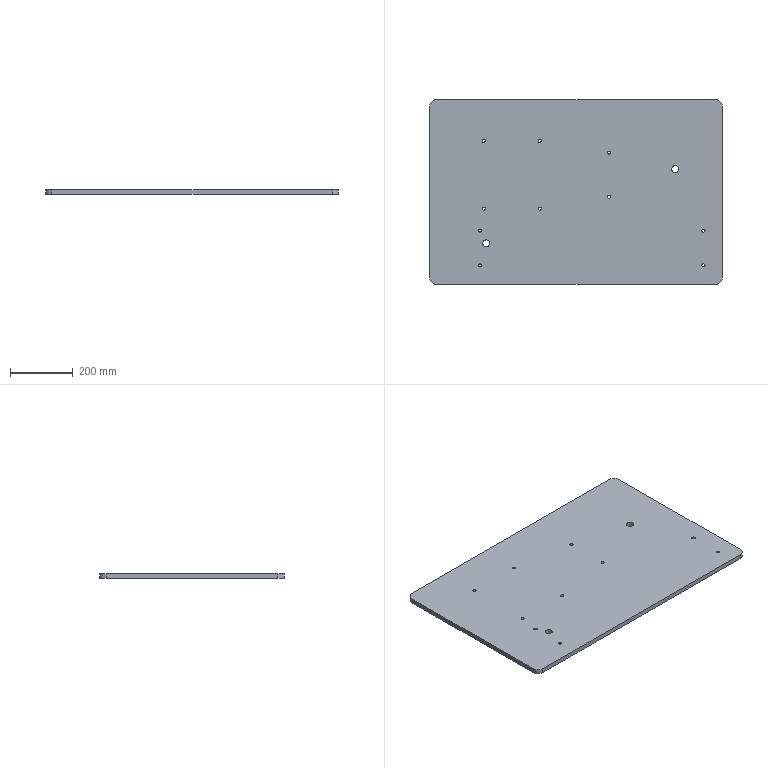Part | SolidWorks | features Extrusion 1 | 1 solid | 34 faces | box 930 x 586 x 15 mm | volume 8146365 mm3 | cylinder 28 | plane 6 | commonest cylinder face diameters 10 x20 22 x4 40 x4
STEP:
#1=CARTESIAN_POINT('',(-296.,-163.,15.));
#2=VERTEX_POINT('',#1);
#3=CARTESIAN_POINT('',(-274.,-163.,15.));
#4=VERTEX_POINT('',#3);
#5=CARTESIAN_POINT('',(-285.,-163.,15.));
#6=DIRECTION('',(0.,0.,1.));
#7=DIRECTION('',(1.,0.,0.));
#8=AXIS2_PLACEMENT_3D('',#5,#6,#7);
#9=CIRCLE('',#8,11.);
#10=EDGE_CURVE('',#2,#4,#9,.T.);
#11=ORIENTED_EDGE('',*,*,#10,.T.);
#12=CARTESIAN_POINT('',(-274.,-163.,0.));
#13=VERTEX_POINT('',#12);
#14=CARTESIAN_POINT('',(-274.,-163.,15.));
#15=DIRECTION('',(0.,0.,-1.));
#16=VECTOR('',#15,1000.);
#17=LINE('',#14,#16);
#18=EDGE_CURVE('',#4,#13,#17,.T.);
#19=ORIENTED_EDGE('',*,*,#18,.T.);
#20=CARTESIAN_POINT('',(-296.,-163.,0.));
#21=VERTEX_POINT('',#20);
#22=CARTESIAN_POINT('',(-285.,-163.,0.));
#23=DIRECTION('',(0.,0.,1.));
#24=DIRECTION('',(1.,0.,0.));
#25=AXIS2_PLACEMENT_3D('',#22,#23,#24);
#26=CIRCLE('',#25,11.);
#27=EDGE_CURVE('',#21,#13,#26,.T.);
#28=ORIENTED_EDGE('',*,*,#27,.F.);
#29=CARTESIAN_POINT('',(-296.,-163.,15.));
#30=DIRECTION('',(0.,0.,-1.));
#31=VECTOR('',#30,1000.);
#32=LINE('',#29,#31);
#33=EDGE_CURVE('',#2,#21,#32,.T.);
#34=ORIENTED_EDGE('',*,*,#33,.F.);
#35=EDGE_LOOP('',(#11,#19,#28,#34));
#36=FACE_OUTER_BOUND('',#35,.T.);
#37=CARTESIAN_POINT('',(-285.,-163.,15.));
#38=DIRECTION('',(0.,0.,-1.));
#39=DIRECTION('',(-1.,0.,0.));
#40=AXIS2_PLACEMENT_3D('',#37,#38,#39);
#41=CYLINDRICAL_SURFACE('',#40,11.);
#42=ADVANCED_FACE('',(#36),#41,.F.);
#43=CARTESIAN_POINT('',(304.,72.5,15.));
#44=VERTEX_POINT('',#43);
#45=CARTESIAN_POINT('',(326.,72.5,15.));
#46=VERTEX_POINT('',#45);
#47=CARTESIAN_POINT('',(315.,72.5,15.));
#48=DIRECTION('',(0.,0.,1.));
#49=DIRECTION('',(1.,0.,0.));
#50=AXIS2_PLACEMENT_3D('',#47,#48,#49);
#51=CIRCLE('',#50,11.);
#52=EDGE_CURVE('',#44,#46,#51,.T.);
#53=ORIENTED_EDGE('',*,*,#52,.T.);
#54=CARTESIAN_POINT('',(326.,72.5,0.));
#55=VERTEX_POINT('',#54);
#56=CARTESIAN_POINT('',(326.,72.5,15.));
#57=DIRECTION('',(0.,0.,-1.));
#58=VECTOR('',#57,1000.);
#59=LINE('',#56,#58);
#60=EDGE_CURVE('',#46,#55,#59,.T.);
#61=ORIENTED_EDGE('',*,*,#60,.T.);
#62=CARTESIAN_POINT('',(304.,72.5,0.));
#63=VERTEX_POINT('',#62);
#64=CARTESIAN_POINT('',(315.,72.5,0.));
#65=DIRECTION('',(0.,0.,1.));
#66=DIRECTION('',(1.,0.,0.));
#67=AXIS2_PLACEMENT_3D('',#64,#65,#66);
#68=CIRCLE('',#67,11.);
#69=EDGE_CURVE('',#63,#55,#68,.T.);
#70=ORIENTED_EDGE('',*,*,#69,.F.);
#71=CARTESIAN_POINT('',(304.,72.5,15.));
#72=DIRECTION('',(0.,0.,-1.));
#73=VECTOR('',#72,1000.);
#74=LINE('',#71,#73);
#75=EDGE_CURVE('',#44,#63,#74,.T.);
#76=ORIENTED_EDGE('',*,*,#75,.F.);
#77=EDGE_LOOP('',(#53,#61,#70,#76));
#78=FACE_OUTER_BOUND('',#77,.T.);
#79=CARTESIAN_POINT('',(315.,72.5,15.));
#80=DIRECTION('',(0.,0.,-1.));
#81=DIRECTION('',(-1.,0.,0.));
#82=AXIS2_PLACEMENT_3D('',#79,#80,#81);
#83=CYLINDRICAL_SURFACE('',#82,11.);
#84=ADVANCED_FACE('',(#78),#83,.F.);
#85=CARTESIAN_POINT('',(400.,-123.,15.));
#86=VERTEX_POINT('',#85);
#87=CARTESIAN_POINT('',(410.,-123.,15.));
#88=VERTEX_POINT('',#87);
#89=CARTESIAN_POINT('',(405.,-123.,15.));
#90=DIRECTION('',(0.,0.,1.));
#91=DIRECTION('',(-1.,0.,0.));
#92=AXIS2_PLACEMENT_3D('',#89,#90,#91);
#93=CIRCLE('',#92,5.);
#94=EDGE_CURVE('',#86,#88,#93,.T.);
#95=ORIENTED_EDGE('',*,*,#94,.T.);
#96=CARTESIAN_POINT('',(410.,-123.,0.));
#97=VERTEX_POINT('',#96);
#98=CARTESIAN_POINT('',(410.,-123.,15.));
#99=DIRECTION('',(0.,0.,-1.));
#100=VECTOR('',#99,1000.);
#101=LINE('',#98,#100);
#102=EDGE_CURVE('',#88,#97,#101,.T.);
#103=ORIENTED_EDGE('',*,*,#102,.T.);
#104=CARTESIAN_POINT('',(400.,-123.,0.));
#105=VERTEX_POINT('',#104);
#106=CARTESIAN_POINT('',(405.,-123.,0.));
#107=DIRECTION('',(0.,0.,1.));
#108=DIRECTION('',(-1.,0.,0.));
#109=AXIS2_PLACEMENT_3D('',#106,#107,#108);
#110=CIRCLE('',#109,5.);
#111=EDGE_CURVE('',#105,#97,#110,.T.);
#112=ORIENTED_EDGE('',*,*,#111,.F.);
#113=CARTESIAN_POINT('',(400.,-123.,15.));
#114=DIRECTION('',(0.,0.,-1.));
#115=VECTOR('',#114,1000.);
#116=LINE('',#113,#115);
#117=EDGE_CURVE('',#86,#105,#116,.T.);
#118=ORIENTED_EDGE('',*,*,#117,.F.);
#119=EDGE_LOOP('',(#95,#103,#112,#118));
#120=FACE_OUTER_BOUND('',#119,.T.);
#121=CARTESIAN_POINT('',(405.,-123.,15.));
#122=DIRECTION('',(0.,0.,-1.));
#123=DIRECTION('',(-1.,0.,0.));
#124=AXIS2_PLACEMENT_3D('',#121,#122,#123);
#125=CYLINDRICAL_SURFACE('',#124,5.);
#126=ADVANCED_FACE('',(#120),#125,.F.);
#127=CARTESIAN_POINT('',(400.,-233.,15.));
#128=VERTEX_POINT('',#127);
#129=CARTESIAN_POINT('',(410.,-233.,15.));
#130=VERTEX_POINT('',#129);
#131=CARTESIAN_POINT('',(405.,-233.,15.));
#132=DIRECTION('',(0.,0.,1.));
#133=DIRECTION('',(1.,0.,0.));
#134=AXIS2_PLACEMENT_3D('',#131,#132,#133);
#135=CIRCLE('',#134,5.);
#136=EDGE_CURVE('',#128,#130,#135,.T.);
#137=ORIENTED_EDGE('',*,*,#136,.T.);
#138=CARTESIAN_POINT('',(410.,-233.,0.));
#139=VERTEX_POINT('',#138);
#140=CARTESIAN_POINT('',(410.,-233.,15.));
#141=DIRECTION('',(0.,0.,-1.));
#142=VECTOR('',#141,1000.);
#143=LINE('',#140,#142);
#144=EDGE_CURVE('',#130,#139,#143,.T.);
#145=ORIENTED_EDGE('',*,*,#144,.T.);
#146=CARTESIAN_POINT('',(400.,-233.,0.));
#147=VERTEX_POINT('',#146);
#148=CARTESIAN_POINT('',(405.,-233.,0.));
#149=DIRECTION('',(0.,0.,1.));
#150=DIRECTION('',(1.,0.,0.));
#151=AXIS2_PLACEMENT_3D('',#148,#149,#150);
#152=CIRCLE('',#151,5.);
#153=EDGE_CURVE('',#147,#139,#152,.T.);
#154=ORIENTED_EDGE('',*,*,#153,.F.);
#155=CARTESIAN_POINT('',(400.,-233.,15.));
#156=DIRECTION('',(0.,0.,-1.));
#157=VECTOR('',#156,1000.);
#158=LINE('',#155,#157);
#159=EDGE_CURVE('',#128,#147,#158,.T.);
#160=ORIENTED_EDGE('',*,*,#159,.F.);
#161=EDGE_LOOP('',(#137,#145,#154,#160));
#162=FACE_OUTER_BOUND('',#161,.T.);
#163=CARTESIAN_POINT('',(405.,-233.,15.));
#164=DIRECTION('',(0.,0.,-1.));
#165=DIRECTION('',(-1.,0.,0.));
#166=AXIS2_PLACEMENT_3D('',#163,#164,#165);
#167=CYLINDRICAL_SURFACE('',#166,5.);
#168=ADVANCED_FACE('',(#162),#167,.F.);
#169=CARTESIAN_POINT('',(-310.,-233.,15.));
#170=VERTEX_POINT('',#169);
#171=CARTESIAN_POINT('',(-300.,-233.,15.));
#172=VERTEX_POINT('',#171);
#173=CARTESIAN_POINT('',(-305.,-233.,15.));
#174=DIRECTION('',(0.,0.,1.));
#175=DIRECTION('',(-1.,0.,0.));
#176=AXIS2_PLACEMENT_3D('',#173,#174,#175);
#177=CIRCLE('',#176,5.);
#178=EDGE_CURVE('',#170,#172,#177,.T.);
#179=ORIENTED_EDGE('',*,*,#178,.T.);
#180=CARTESIAN_POINT('',(-300.,-233.,0.));
#181=VERTEX_POINT('',#180);
#182=CARTESIAN_POINT('',(-300.,-233.,15.));
#183=DIRECTION('',(0.,0.,-1.));
#184=VECTOR('',#183,1000.);
#185=LINE('',#182,#184);
#186=EDGE_CURVE('',#172,#181,#185,.T.);
#187=ORIENTED_EDGE('',*,*,#186,.T.);
#188=CARTESIAN_POINT('',(-310.,-233.,0.));
#189=VERTEX_POINT('',#188);
#190=CARTESIAN_POINT('',(-305.,-233.,0.));
#191=DIRECTION('',(0.,0.,1.));
#192=DIRECTION('',(-1.,0.,0.));
#193=AXIS2_PLACEMENT_3D('',#190,#191,#192);
#194=CIRCLE('',#193,5.);
#195=EDGE_CURVE('',#189,#181,#194,.T.);
#196=ORIENTED_EDGE('',*,*,#195,.F.);
#197=CARTESIAN_POINT('',(-310.,-233.,15.));
#198=DIRECTION('',(0.,0.,-1.));
#199=VECTOR('',#198,1000.);
#200=LINE('',#197,#199);
#201=EDGE_CURVE('',#170,#189,#200,.T.);
#202=ORIENTED_EDGE('',*,*,#201,.F.);
#203=EDGE_LOOP('',(#179,#187,#196,#202));
#204=FACE_OUTER_BOUND('',#203,.T.);
#205=CARTESIAN_POINT('',(-305.,-233.,15.));
#206=DIRECTION('',(0.,0.,-1.));
#207=DIRECTION('',(-1.,0.,0.));
#208=AXIS2_PLACEMENT_3D('',#205,#206,#207);
#209=CYLINDRICAL_SURFACE('',#208,5.);
#210=ADVANCED_FACE('',(#204),#209,.F.);
#211=CARTESIAN_POINT('',(-310.,-123.,15.));
#212=VERTEX_POINT('',#211);
#213=CARTESIAN_POINT('',(-300.,-123.,15.));
#214=VERTEX_POINT('',#213);
#215=CARTESIAN_POINT('',(-305.,-123.,15.));
#216=DIRECTION('',(0.,0.,1.));
#217=DIRECTION('',(1.,0.,0.));
#218=AXIS2_PLACEMENT_3D('',#215,#216,#217);
#219=CIRCLE('',#218,5.);
#220=EDGE_CURVE('',#212,#214,#219,.T.);
#221=ORIENTED_EDGE('',*,*,#220,.T.);
#222=CARTESIAN_POINT('',(-300.,-123.,0.));
#223=VERTEX_POINT('',#222);
#224=CARTESIAN_POINT('',(-300.,-123.,15.));
#225=DIRECTION('',(0.,0.,-1.));
#226=VECTOR('',#225,1000.);
#227=LINE('',#224,#226);
#228=EDGE_CURVE('',#214,#223,#227,.T.);
#229=ORIENTED_EDGE('',*,*,#228,.T.);
#230=CARTESIAN_POINT('',(-310.,-123.,0.));
#231=VERTEX_POINT('',#230);
#232=CARTESIAN_POINT('',(-305.,-123.,0.));
#233=DIRECTION('',(0.,0.,1.));
#234=DIRECTION('',(1.,0.,0.));
#235=AXIS2_PLACEMENT_3D('',#232,#233,#234);
#236=CIRCLE('',#235,5.);
#237=EDGE_CURVE('',#231,#223,#236,.T.);
#238=ORIENTED_EDGE('',*,*,#237,.F.);
#239=CARTESIAN_POINT('',(-310.,-123.,15.));
#240=DIRECTION('',(0.,0.,-1.));
#241=VECTOR('',#240,1000.);
#242=LINE('',#239,#241);
#243=EDGE_CURVE('',#212,#231,#242,.T.);
#244=ORIENTED_EDGE('',*,*,#243,.F.);
#245=EDGE_LOOP('',(#221,#229,#238,#244));
#246=FACE_OUTER_BOUND('',#245,.T.);
#247=CARTESIAN_POINT('',(-305.,-123.,15.));
#248=DIRECTION('',(0.,0.,-1.));
#249=DIRECTION('',(-1.,0.,0.));
#250=AXIS2_PLACEMENT_3D('',#247,#248,#249);
#251=CYLINDRICAL_SURFACE('',#250,5.);
#252=ADVANCED_FACE('',(#246),#251,.F.);
#253=CARTESIAN_POINT('',(100.,-15.,15.));
#254=VERTEX_POINT('',#253);
#255=CARTESIAN_POINT('',(110.,-15.,15.));
#256=VERTEX_POINT('',#255);
#257=CARTESIAN_POINT('',(105.,-15.,15.));
#258=DIRECTION('',(0.,0.,1.));
#259=DIRECTION('',(1.,0.,0.));
#260=AXIS2_PLACEMENT_3D('',#257,#258,#259);
#261=CIRCLE('',#260,5.);
#262=EDGE_CURVE('',#254,#256,#261,.T.);
#263=ORIENTED_EDGE('',*,*,#262,.T.);
#264=CARTESIAN_POINT('',(110.,-15.,0.));
#265=VERTEX_POINT('',#264);
#266=CARTESIAN_POINT('',(110.,-15.,15.));
#267=DIRECTION('',(0.,0.,-1.));
#268=VECTOR('',#267,1000.);
#269=LINE('',#266,#268);
#270=EDGE_CURVE('',#256,#265,#269,.T.);
#271=ORIENTED_EDGE('',*,*,#270,.T.);
#272=CARTESIAN_POINT('',(100.,-15.,0.));
#273=VERTEX_POINT('',#272);
#274=CARTESIAN_POINT('',(105.,-15.,0.));
#275=DIRECTION('',(0.,0.,1.));
#276=DIRECTION('',(1.,0.,0.));
#277=AXIS2_PLACEMENT_3D('',#274,#275,#276);
#278=CIRCLE('',#277,5.);
#279=EDGE_CURVE('',#273,#265,#278,.T.);
#280=ORIENTED_EDGE('',*,*,#279,.F.);
#281=CARTESIAN_POINT('',(100.,-15.,15.));
#282=DIRECTION('',(0.,0.,-1.));
#283=VECTOR('',#282,1000.);
#284=LINE('',#281,#283);
#285=EDGE_CURVE('',#254,#273,#284,.T.);
#286=ORIENTED_EDGE('',*,*,#285,.F.);
#287=EDGE_LOOP('',(#263,#271,#280,#286));
#288=FACE_OUTER_BOUND('',#287,.T.);
#289=CARTESIAN_POINT('',(105.,-15.,15.));
#290=DIRECTION('',(0.,0.,-1.));
#291=DIRECTION('',(-1.,0.,0.));
#292=AXIS2_PLACEMENT_3D('',#289,#290,#291);
#293=CYLINDRICAL_SURFACE('',#292,5.);
#294=ADVANCED_FACE('',(#288),#293,.F.);
#295=CARTESIAN_POINT('',(100.,125.,15.));
#296=VERTEX_POINT('',#295);
#297=CARTESIAN_POINT('',(110.,125.,15.));
#298=VERTEX_POINT('',#297);
#299=CARTESIAN_POINT('',(105.,125.,15.));
#300=DIRECTION('',(0.,0.,1.));
#301=DIRECTION('',(-1.,0.,0.));
#302=AXIS2_PLACEMENT_3D('',#299,#300,#301);
#303=CIRCLE('',#302,5.);
#304=EDGE_CURVE('',#296,#298,#303,.T.);
#305=ORIENTED_EDGE('',*,*,#304,.T.);
#306=CARTESIAN_POINT('',(110.,125.,0.));
#307=VERTEX_POINT('',#306);
#308=CARTESIAN_POINT('',(110.,125.,15.));
#309=DIRECTION('',(0.,0.,-1.));
#310=VECTOR('',#309,1000.);
#311=LINE('',#308,#310);
#312=EDGE_CURVE('',#298,#307,#311,.T.);
#313=ORIENTED_EDGE('',*,*,#312,.T.);
#314=CARTESIAN_POINT('',(100.,125.,0.));
#315=VERTEX_POINT('',#314);
#316=CARTESIAN_POINT('',(105.,125.,0.));
#317=DIRECTION('',(0.,0.,1.));
#318=DIRECTION('',(-1.,0.,0.));
#319=AXIS2_PLACEMENT_3D('',#316,#317,#318);
#320=CIRCLE('',#319,5.);
#321=EDGE_CURVE('',#315,#307,#320,.T.);
#322=ORIENTED_EDGE('',*,*,#321,.F.);
#323=CARTESIAN_POINT('',(100.,125.,15.));
#324=DIRECTION('',(0.,0.,-1.));
#325=VECTOR('',#324,1000.);
#326=LINE('',#323,#325);
#327=EDGE_CURVE('',#296,#315,#326,.T.);
#328=ORIENTED_EDGE('',*,*,#327,.F.);
#329=EDGE_LOOP('',(#305,#313,#322,#328));
#330=FACE_OUTER_BOUND('',#329,.T.);
#331=CARTESIAN_POINT('',(105.,125.,15.));
#332=DIRECTION('',(0.,0.,-1.));
#333=DIRECTION('',(-1.,0.,0.));
#334=AXIS2_PLACEMENT_3D('',#331,#332,#333);
#335=CYLINDRICAL_SURFACE('',#334,5.);
#336=ADVANCED_FACE('',(#330),#335,.F.);
#337=CARTESIAN_POINT('',(-298.,-53.,15.));
#338=VERTEX_POINT('',#337);
#339=CARTESIAN_POINT('',(-288.,-53.,15.));
#340=VERTEX_POINT('',#339);
#341=CARTESIAN_POINT('',(-293.,-53.,15.));
#342=DIRECTION('',(0.,0.,1.));
#343=DIRECTION('',(-1.,0.,0.));
#344=AXIS2_PLACEMENT_3D('',#341,#342,#343);
#345=CIRCLE('',#344,5.);
#346=EDGE_CURVE('',#338,#340,#345,.T.);
#347=ORIENTED_EDGE('',*,*,#346,.T.);
#348=CARTESIAN_POINT('',(-288.,-53.,0.));
#349=VERTEX_POINT('',#348);
#350=CARTESIAN_POINT('',(-288.,-53.,15.));
#351=DIRECTION('',(0.,0.,-1.));
#352=VECTOR('',#351,1000.);
#353=LINE('',#350,#352);
#354=EDGE_CURVE('',#340,#349,#353,.T.);
#355=ORIENTED_EDGE('',*,*,#354,.T.);
#356=CARTESIAN_POINT('',(-298.,-53.,0.));
#357=VERTEX_POINT('',#356);
#358=CARTESIAN_POINT('',(-293.,-53.,0.));
#359=DIRECTION('',(0.,0.,1.));
#360=DIRECTION('',(-1.,0.,0.));
#361=AXIS2_PLACEMENT_3D('',#358,#359,#360);
#362=CIRCLE('',#361,5.);
#363=EDGE_CURVE('',#357,#349,#362,.T.);
#364=ORIENTED_EDGE('',*,*,#363,.F.);
#365=CARTESIAN_POINT('',(-298.,-53.,15.));
#366=DIRECTION('',(0.,0.,-1.));
#367=VECTOR('',#366,1000.);
#368=LINE('',#365,#367);
#369=EDGE_CURVE('',#338,#357,#368,.T.);
#370=ORIENTED_EDGE('',*,*,#369,.F.);
#371=EDGE_LOOP('',(#347,#355,#364,#370));
#372=FACE_OUTER_BOUND('',#371,.T.);
#373=CARTESIAN_POINT('',(-293.,-53.,15.));
#374=DIRECTION('',(0.,0.,-1.));
#375=DIRECTION('',(-1.,0.,0.));
#376=AXIS2_PLACEMENT_3D('',#373,#374,#375);
#377=CYLINDRICAL_SURFACE('',#376,5.);
#378=ADVANCED_FACE('',(#372),#377,.F.);
#379=CARTESIAN_POINT('',(-120.,-53.,15.));
#380=VERTEX_POINT('',#379);
#381=CARTESIAN_POINT('',(-110.,-53.,15.));
#382=VERTEX_POINT('',#381);
#383=CARTESIAN_POINT('',(-115.,-53.,15.));
#384=DIRECTION('',(0.,0.,1.));
#385=DIRECTION('',(-1.,0.,0.));
#386=AXIS2_PLACEMENT_3D('',#383,#384,#385);
#387=CIRCLE('',#386,5.);
#388=EDGE_CURVE('',#380,#382,#387,.T.);
#389=ORIENTED_EDGE('',*,*,#388,.T.);
#390=CARTESIAN_POINT('',(-110.,-53.,0.));
#391=VERTEX_POINT('',#390);
#392=CARTESIAN_POINT('',(-110.,-53.,15.));
#393=DIRECTION('',(0.,0.,-1.));
#394=VECTOR('',#393,1000.);
#395=LINE('',#392,#394);
#396=EDGE_CURVE('',#382,#391,#395,.T.);
#397=ORIENTED_EDGE('',*,*,#396,.T.);
#398=CARTESIAN_POINT('',(-120.,-53.,0.));
#399=VERTEX_POINT('',#398);
#400=CARTESIAN_POINT('',(-115.,-53.,0.));
#401=DIRECTION('',(0.,0.,1.));
#402=DIRECTION('',(-1.,0.,0.));
#403=AXIS2_PLACEMENT_3D('',#400,#401,#402);
#404=CIRCLE('',#403,5.);
#405=EDGE_CURVE('',#399,#391,#404,.T.);
#406=ORIENTED_EDGE('',*,*,#405,.F.);
#407=CARTESIAN_POINT('',(-120.,-53.,15.));
#408=DIRECTION('',(0.,0.,-1.));
#409=VECTOR('',#408,1000.);
#410=LINE('',#407,#409);
#411=EDGE_CURVE('',#380,#399,#410,.T.);
#412=ORIENTED_EDGE('',*,*,#411,.F.);
#413=EDGE_LOOP('',(#389,#397,#406,#412));
#414=FACE_OUTER_BOUND('',#413,.T.);
#415=CARTESIAN_POINT('',(-115.,-53.,15.));
#416=DIRECTION('',(0.,0.,-1.));
#417=DIRECTION('',(-1.,0.,0.));
#418=AXIS2_PLACEMENT_3D('',#415,#416,#417);
#419=CYLINDRICAL_SURFACE('',#418,5.);
#420=ADVANCED_FACE('',(#414),#419,.F.);
#421=CARTESIAN_POINT('',(-298.,163.,15.));
#422=VERTEX_POINT('',#421);
#423=CARTESIAN_POINT('',(-288.,163.,15.));
#424=VERTEX_POINT('',#423);
#425=CARTESIAN_POINT('',(-293.,163.,15.));
#426=DIRECTION('',(0.,0.,1.));
#427=DIRECTION('',(1.,0.,0.));
#428=AXIS2_PLACEMENT_3D('',#425,#426,#427);
#429=CIRCLE('',#428,5.);
#430=EDGE_CURVE('',#422,#424,#429,.T.);
#431=ORIENTED_EDGE('',*,*,#430,.T.);
#432=CARTESIAN_POINT('',(-288.,163.,0.));
#433=VERTEX_POINT('',#432);
#434=CARTESIAN_POINT('',(-288.,163.,15.));
#435=DIRECTION('',(0.,0.,-1.));
#436=VECTOR('',#435,1000.);
#437=LINE('',#434,#436);
#438=EDGE_CURVE('',#424,#433,#437,.T.);
#439=ORIENTED_EDGE('',*,*,#438,.T.);
#440=CARTESIAN_POINT('',(-298.,163.,0.));
#441=VERTEX_POINT('',#440);
#442=CARTESIAN_POINT('',(-293.,163.,0.));
#443=DIRECTION('',(0.,0.,1.));
#444=DIRECTION('',(1.,0.,0.));
#445=AXIS2_PLACEMENT_3D('',#442,#443,#444);
#446=CIRCLE('',#445,5.);
#447=EDGE_CURVE('',#441,#433,#446,.T.);
#448=ORIENTED_EDGE('',*,*,#447,.F.);
#449=CARTESIAN_POINT('',(-298.,163.,15.));
#450=DIRECTION('',(0.,0.,-1.));
#451=VECTOR('',#450,1000.);
#452=LINE('',#449,#451);
#453=EDGE_CURVE('',#422,#441,#452,.T.);
#454=ORIENTED_EDGE('',*,*,#453,.F.);
#455=EDGE_LOOP('',(#431,#439,#448,#454));
#456=FACE_OUTER_BOUND('',#455,.T.);
#457=CARTESIAN_POINT('',(-293.,163.,15.));
#458=DIRECTION('',(0.,0.,-1.));
#459=DIRECTION('',(-1.,0.,0.));
#460=AXIS2_PLACEMENT_3D('',#457,#458,#459);
#461=CYLINDRICAL_SURFACE('',#460,5.);
#462=ADVANCED_FACE('',(#456),#461,.F.);
#463=CARTESIAN_POINT('',(-120.,163.,15.));
#464=VERTEX_POINT('',#463);
#465=CARTESIAN_POINT('',(-110.,163.,15.));
#466=VERTEX_POINT('',#465);
#467=CARTESIAN_POINT('',(-115.,163.,15.));
#468=DIRECTION('',(0.,0.,1.));
#469=DIRECTION('',(1.,0.,0.));
#470=AXIS2_PLACEMENT_3D('',#467,#468,#469);
#471=CIRCLE('',#470,5.);
#472=EDGE_CURVE('',#464,#466,#471,.T.);
#473=ORIENTED_EDGE('',*,*,#472,.T.);
#474=CARTESIAN_POINT('',(-110.,163.,0.));
#475=VERTEX_POINT('',#474);
#476=CARTESIAN_POINT('',(-110.,163.,15.));
#477=DIRECTION('',(0.,0.,-1.));
#478=VECTOR('',#477,1000.);
#479=LINE('',#476,#478);
#480=EDGE_CURVE('',#466,#475,#479,.T.);
#481=ORIENTED_EDGE('',*,*,#480,.T.);
#482=CARTESIAN_POINT('',(-120.,163.,0.));
#483=VERTEX_POINT('',#482);
#484=CARTESIAN_POINT('',(-115.,163.,0.));
#485=DIRECTION('',(0.,0.,1.));
#486=DIRECTION('',(1.,0.,0.));
#487=AXIS2_PLACEMENT_3D('',#484,#485,#486);
#488=CIRCLE('',#487,5.);
#489=EDGE_CURVE('',#483,#475,#488,.T.);
#490=ORIENTED_EDGE('',*,*,#489,.F.);
#491=CARTESIAN_POINT('',(-120.,163.,15.));
#492=DIRECTION('',(0.,0.,-1.));
#493=VECTOR('',#492,1000.);
#494=LINE('',#491,#493);
#495=EDGE_CURVE('',#464,#483,#494,.T.);
#496=ORIENTED_EDGE('',*,*,#495,.F.);
#497=EDGE_LOOP('',(#473,#481,#490,#496));
#498=FACE_OUTER_BOUND('',#497,.T.);
#499=CARTESIAN_POINT('',(-115.,163.,15.));
#500=DIRECTION('',(0.,0.,-1.));
#501=DIRECTION('',(-1.,0.,0.));
#502=AXIS2_PLACEMENT_3D('',#499,#500,#501);
#503=CYLINDRICAL_SURFACE('',#502,5.);
#504=ADVANCED_FACE('',(#498),#503,.F.);
#505=CARTESIAN_POINT('',(-465.,-273.,15.));
#506=VERTEX_POINT('',#505);
#507=CARTESIAN_POINT('',(-445.,-293.,15.));
#508=VERTEX_POINT('',#507);
#509=CARTESIAN_POINT('',(-445.,-273.,15.));
#510=DIRECTION('',(0.,0.,1.));
#511=DIRECTION('',(-1.,0.,0.));
#512=AXIS2_PLACEMENT_3D('',#509,#510,#511);
#513=CIRCLE('',#512,20.);
#514=EDGE_CURVE('',#506,#508,#513,.T.);
#515=ORIENTED_EDGE('',*,*,#514,.T.);
#516=CARTESIAN_POINT('',(445.,-293.,15.));
#517=VERTEX_POINT('',#516);
#518=CARTESIAN_POINT('',(-445.,-293.,15.));
#519=DIRECTION('',(1.,0.,0.));
#520=VECTOR('',#519,1000.);
#521=LINE('',#518,#520);
#522=EDGE_CURVE('',#508,#517,#521,.T.);
#523=ORIENTED_EDGE('',*,*,#522,.T.);
#524=CARTESIAN_POINT('',(465.,-273.,15.));
#525=VERTEX_POINT('',#524);
#526=CARTESIAN_POINT('',(445.,-273.,15.));
#527=DIRECTION('',(0.,0.,1.));
#528=DIRECTION('',(-1.,0.,0.));
#529=AXIS2_PLACEMENT_3D('',#526,#527,#528);
#530=CIRCLE('',#529,20.);
#531=EDGE_CURVE('',#517,#525,#530,.T.);
#532=ORIENTED_EDGE('',*,*,#531,.T.);
#533=CARTESIAN_POINT('',(465.,273.,15.));
#534=VERTEX_POINT('',#533);
#535=CARTESIAN_POINT('',(465.,-273.,15.));
#536=DIRECTION('',(0.,1.,0.));
#537=VECTOR('',#536,1000.);
#538=LINE('',#535,#537);
#539=EDGE_CURVE('',#525,#534,#538,.T.);
#540=ORIENTED_EDGE('',*,*,#539,.T.);
#541=CARTESIAN_POINT('',(445.,293.,15.));
#542=VERTEX_POINT('',#541);
#543=CARTESIAN_POINT('',(445.,273.,15.));
#544=DIRECTION('',(0.,0.,1.));
#545=DIRECTION('',(1.,0.,0.));
#546=AXIS2_PLACEMENT_3D('',#543,#544,#545);
#547=CIRCLE('',#546,20.);
#548=EDGE_CURVE('',#534,#542,#547,.T.);
#549=ORIENTED_EDGE('',*,*,#548,.T.);
#550=CARTESIAN_POINT('',(-445.,293.,15.));
#551=VERTEX_POINT('',#550);
#552=CARTESIAN_POINT('',(-445.,293.,15.));
#553=DIRECTION('',(-1.,0.,0.));
#554=VECTOR('',#553,1000.);
#555=LINE('',#552,#554);
#556=EDGE_CURVE('',#542,#551,#555,.T.);
#557=ORIENTED_EDGE('',*,*,#556,.T.);
#558=CARTESIAN_POINT('',(-465.,273.,15.));
#559=VERTEX_POINT('',#558);
#560=CARTESIAN_POINT('',(-445.,273.,15.));
#561=DIRECTION('',(0.,0.,1.));
#562=DIRECTION('',(-1.,0.,0.));
#563=AXIS2_PLACEMENT_3D('',#560,#561,#562);
#564=CIRCLE('',#563,20.);
#565=EDGE_CURVE('',#551,#559,#564,.T.);
#566=ORIENTED_EDGE('',*,*,#565,.T.);
#567=CARTESIAN_POINT('',(-465.,-273.,15.));
#568=DIRECTION('',(0.,-1.,0.));
#569=VECTOR('',#568,1000.);
#570=LINE('',#567,#569);
#571=EDGE_CURVE('',#559,#506,#570,.T.);
#572=ORIENTED_EDGE('',*,*,#571,.T.);
#573=EDGE_LOOP('',(#515,#523,#532,#540,#549,#557,#566,#572));
#574=FACE_OUTER_BOUND('',#573,.T.);
#575=ORIENTED_EDGE('',*,*,#472,.F.);
#576=CARTESIAN_POINT('',(-115.,163.,15.));
#577=DIRECTION('',(0.,0.,1.));
#578=DIRECTION('',(1.,0.,0.));
#579=AXIS2_PLACEMENT_3D('',#576,#577,#578);
#580=CIRCLE('',#579,5.);
#581=EDGE_CURVE('',#466,#464,#580,.T.);
#582=ORIENTED_EDGE('',*,*,#581,.F.);
#583=EDGE_LOOP('',(#575,#582));
#584=FACE_BOUND('',#583,.T.);
#585=ORIENTED_EDGE('',*,*,#430,.F.);
#586=CARTESIAN_POINT('',(-293.,163.,15.));
#587=DIRECTION('',(0.,0.,1.));
#588=DIRECTION('',(1.,0.,0.));
#589=AXIS2_PLACEMENT_3D('',#586,#587,#588);
#590=CIRCLE('',#589,5.);
#591=EDGE_CURVE('',#424,#422,#590,.T.);
#592=ORIENTED_EDGE('',*,*,#591,.F.);
#593=EDGE_LOOP('',(#585,#592));
#594=FACE_BOUND('',#593,.T.);
#595=ORIENTED_EDGE('',*,*,#388,.F.);
#596=CARTESIAN_POINT('',(-115.,-53.,15.));
#597=DIRECTION('',(0.,0.,1.));
#598=DIRECTION('',(-1.,0.,0.));
#599=AXIS2_PLACEMENT_3D('',#596,#597,#598);
#600=CIRCLE('',#599,5.);
#601=EDGE_CURVE('',#382,#380,#600,.T.);
#602=ORIENTED_EDGE('',*,*,#601,.F.);
#603=EDGE_LOOP('',(#595,#602));
#604=FACE_BOUND('',#603,.T.);
#605=ORIENTED_EDGE('',*,*,#346,.F.);
#606=CARTESIAN_POINT('',(-293.,-53.,15.));
#607=DIRECTION('',(0.,0.,1.));
#608=DIRECTION('',(-1.,0.,0.));
#609=AXIS2_PLACEMENT_3D('',#606,#607,#608);
#610=CIRCLE('',#609,5.);
#611=EDGE_CURVE('',#340,#338,#610,.T.);
#612=ORIENTED_EDGE('',*,*,#611,.F.);
#613=EDGE_LOOP('',(#605,#612));
#614=FACE_BOUND('',#613,.T.);
#615=ORIENTED_EDGE('',*,*,#304,.F.);
#616=CARTESIAN_POINT('',(105.,125.,15.));
#617=DIRECTION('',(0.,0.,1.));
#618=DIRECTION('',(-1.,0.,0.));
#619=AXIS2_PLACEMENT_3D('',#616,#617,#618);
#620=CIRCLE('',#619,5.);
#621=EDGE_CURVE('',#298,#296,#620,.T.);
#622=ORIENTED_EDGE('',*,*,#621,.F.);
#623=EDGE_LOOP('',(#615,#622));
#624=FACE_BOUND('',#623,.T.);
#625=ORIENTED_EDGE('',*,*,#262,.F.);
#626=CARTESIAN_POINT('',(105.,-15.,15.));
#627=DIRECTION('',(0.,0.,1.));
#628=DIRECTION('',(1.,0.,0.));
#629=AXIS2_PLACEMENT_3D('',#626,#627,#628);
#630=CIRCLE('',#629,5.);
#631=EDGE_CURVE('',#256,#254,#630,.T.);
#632=ORIENTED_EDGE('',*,*,#631,.F.);
#633=EDGE_LOOP('',(#625,#632));
#634=FACE_BOUND('',#633,.T.);
#635=ORIENTED_EDGE('',*,*,#220,.F.);
#636=CARTESIAN_POINT('',(-305.,-123.,15.));
#637=DIRECTION('',(0.,0.,1.));
#638=DIRECTION('',(1.,0.,0.));
#639=AXIS2_PLACEMENT_3D('',#636,#637,#638);
#640=CIRCLE('',#639,5.);
#641=EDGE_CURVE('',#214,#212,#640,.T.);
#642=ORIENTED_EDGE('',*,*,#641,.F.);
#643=EDGE_LOOP('',(#635,#642));
#644=FACE_BOUND('',#643,.T.);
#645=ORIENTED_EDGE('',*,*,#178,.F.);
#646=CARTESIAN_POINT('',(-305.,-233.,15.));
#647=DIRECTION('',(0.,0.,1.));
#648=DIRECTION('',(-1.,0.,0.));
#649=AXIS2_PLACEMENT_3D('',#646,#647,#648);
#650=CIRCLE('',#649,5.);
#651=EDGE_CURVE('',#172,#170,#650,.T.);
#652=ORIENTED_EDGE('',*,*,#651,.F.);
#653=EDGE_LOOP('',(#645,#652));
#654=FACE_BOUND('',#653,.T.);
#655=ORIENTED_EDGE('',*,*,#136,.F.);
#656=CARTESIAN_POINT('',(405.,-233.,15.));
#657=DIRECTION('',(0.,0.,1.));
#658=DIRECTION('',(1.,0.,0.));
#659=AXIS2_PLACEMENT_3D('',#656,#657,#658);
#660=CIRCLE('',#659,5.);
#661=EDGE_CURVE('',#130,#128,#660,.T.);
#662=ORIENTED_EDGE('',*,*,#661,.F.);
#663=EDGE_LOOP('',(#655,#662));
#664=FACE_BOUND('',#663,.T.);
#665=ORIENTED_EDGE('',*,*,#94,.F.);
#666=CARTESIAN_POINT('',(405.,-123.,15.));
#667=DIRECTION('',(0.,0.,1.));
#668=DIRECTION('',(-1.,0.,0.));
#669=AXIS2_PLACEMENT_3D('',#666,#667,#668);
#670=CIRCLE('',#669,5.);
#671=EDGE_CURVE('',#88,#86,#670,.T.);
#672=ORIENTED_EDGE('',*,*,#671,.F.);
#673=EDGE_LOOP('',(#665,#672));
#674=FACE_BOUND('',#673,.T.);
#675=ORIENTED_EDGE('',*,*,#52,.F.);
#676=CARTESIAN_POINT('',(315.,72.5,15.));
#677=DIRECTION('',(0.,0.,1.));
#678=DIRECTION('',(1.,0.,0.));
#679=AXIS2_PLACEMENT_3D('',#676,#677,#678);
#680=CIRCLE('',#679,11.);
#681=EDGE_CURVE('',#46,#44,#680,.T.);
#682=ORIENTED_EDGE('',*,*,#681,.F.);
#683=EDGE_LOOP('',(#675,#682));
#684=FACE_BOUND('',#683,.T.);
#685=ORIENTED_EDGE('',*,*,#10,.F.);
#686=CARTESIAN_POINT('',(-285.,-163.,15.));
#687=DIRECTION('',(0.,0.,1.));
#688=DIRECTION('',(1.,0.,0.));
#689=AXIS2_PLACEMENT_3D('',#686,#687,#688);
#690=CIRCLE('',#689,11.);
#691=EDGE_CURVE('',#4,#2,#690,.T.);
#692=ORIENTED_EDGE('',*,*,#691,.F.);
#693=EDGE_LOOP('',(#685,#692));
#694=FACE_BOUND('',#693,.T.);
#695=CARTESIAN_POINT('',(-445.,-273.,15.));
#696=DIRECTION('',(0.,0.,-1.));
#697=DIRECTION('',(-1.,0.,0.));
#698=AXIS2_PLACEMENT_3D('',#695,#696,#697);
#699=PLANE('',#698);
#700=ADVANCED_FACE('',(#574,#584,#594,#604,#614,#624,#634,#644,#654,#664,#674,#684,#694),#699,.F.);
#701=ORIENTED_EDGE('',*,*,#69,.T.);
#702=CARTESIAN_POINT('',(315.,72.5,0.));
#703=DIRECTION('',(0.,0.,1.));
#704=DIRECTION('',(1.,0.,0.));
#705=AXIS2_PLACEMENT_3D('',#702,#703,#704);
#706=CIRCLE('',#705,11.);
#707=EDGE_CURVE('',#55,#63,#706,.T.);
#708=ORIENTED_EDGE('',*,*,#707,.T.);
#709=EDGE_LOOP('',(#701,#708));
#710=FACE_BOUND('',#709,.T.);
#711=ORIENTED_EDGE('',*,*,#153,.T.);
#712=CARTESIAN_POINT('',(405.,-233.,0.));
#713=DIRECTION('',(0.,0.,1.));
#714=DIRECTION('',(1.,0.,0.));
#715=AXIS2_PLACEMENT_3D('',#712,#713,#714);
#716=CIRCLE('',#715,5.);
#717=EDGE_CURVE('',#139,#147,#716,.T.);
#718=ORIENTED_EDGE('',*,*,#717,.T.);
#719=EDGE_LOOP('',(#711,#718));
#720=FACE_BOUND('',#719,.T.);
#721=ORIENTED_EDGE('',*,*,#237,.T.);
#722=CARTESIAN_POINT('',(-305.,-123.,0.));
#723=DIRECTION('',(0.,0.,1.));
#724=DIRECTION('',(1.,0.,0.));
#725=AXIS2_PLACEMENT_3D('',#722,#723,#724);
#726=CIRCLE('',#725,5.);
#727=EDGE_CURVE('',#223,#231,#726,.T.);
#728=ORIENTED_EDGE('',*,*,#727,.T.);
#729=EDGE_LOOP('',(#721,#728));
#730=FACE_BOUND('',#729,.T.);
#731=ORIENTED_EDGE('',*,*,#321,.T.);
#732=CARTESIAN_POINT('',(105.,125.,0.));
#733=DIRECTION('',(0.,0.,1.));
#734=DIRECTION('',(-1.,0.,0.));
#735=AXIS2_PLACEMENT_3D('',#732,#733,#734);
#736=CIRCLE('',#735,5.);
#737=EDGE_CURVE('',#307,#315,#736,.T.);
#738=ORIENTED_EDGE('',*,*,#737,.T.);
#739=EDGE_LOOP('',(#731,#738));
#740=FACE_BOUND('',#739,.T.);
#741=ORIENTED_EDGE('',*,*,#405,.T.);
#742=CARTESIAN_POINT('',(-115.,-53.,0.));
#743=DIRECTION('',(0.,0.,1.));
#744=DIRECTION('',(-1.,0.,0.));
#745=AXIS2_PLACEMENT_3D('',#742,#743,#744);
#746=CIRCLE('',#745,5.);
#747=EDGE_CURVE('',#391,#399,#746,.T.);
#748=ORIENTED_EDGE('',*,*,#747,.T.);
#749=EDGE_LOOP('',(#741,#748));
#750=FACE_BOUND('',#749,.T.);
#751=ORIENTED_EDGE('',*,*,#489,.T.);
#752=CARTESIAN_POINT('',(-115.,163.,0.));
#753=DIRECTION('',(0.,0.,1.));
#754=DIRECTION('',(1.,0.,0.));
#755=AXIS2_PLACEMENT_3D('',#752,#753,#754);
#756=CIRCLE('',#755,5.);
#757=EDGE_CURVE('',#475,#483,#756,.T.);
#758=ORIENTED_EDGE('',*,*,#757,.T.);
#759=EDGE_LOOP('',(#751,#758));
#760=FACE_BOUND('',#759,.T.);
#761=CARTESIAN_POINT('',(-465.,-273.,0.));
#762=VERTEX_POINT('',#761);
#763=CARTESIAN_POINT('',(-445.,-293.,0.));
#764=VERTEX_POINT('',#763);
#765=CARTESIAN_POINT('',(-445.,-273.,0.));
#766=DIRECTION('',(0.,0.,1.));
#767=DIRECTION('',(-1.,0.,0.));
#768=AXIS2_PLACEMENT_3D('',#765,#766,#767);
#769=CIRCLE('',#768,20.);
#770=EDGE_CURVE('',#762,#764,#769,.T.);
#771=ORIENTED_EDGE('',*,*,#770,.F.);
#772=CARTESIAN_POINT('',(-465.,273.,0.));
#773=VERTEX_POINT('',#772);
#774=CARTESIAN_POINT('',(-465.,-273.,0.));
#775=DIRECTION('',(0.,-1.,0.));
#776=VECTOR('',#775,1000.);
#777=LINE('',#774,#776);
#778=EDGE_CURVE('',#773,#762,#777,.T.);
#779=ORIENTED_EDGE('',*,*,#778,.F.);
#780=CARTESIAN_POINT('',(-445.,293.,0.));
#781=VERTEX_POINT('',#780);
#782=CARTESIAN_POINT('',(-445.,273.,0.));
#783=DIRECTION('',(0.,0.,1.));
#784=DIRECTION('',(-1.,0.,0.));
#785=AXIS2_PLACEMENT_3D('',#782,#783,#784);
#786=CIRCLE('',#785,20.);
#787=EDGE_CURVE('',#781,#773,#786,.T.);
#788=ORIENTED_EDGE('',*,*,#787,.F.);
#789=CARTESIAN_POINT('',(445.,293.,0.));
#790=VERTEX_POINT('',#789);
#791=CARTESIAN_POINT('',(-445.,293.,0.));
#792=DIRECTION('',(-1.,0.,0.));
#793=VECTOR('',#792,1000.);
#794=LINE('',#791,#793);
#795=EDGE_CURVE('',#790,#781,#794,.T.);
#796=ORIENTED_EDGE('',*,*,#795,.F.);
#797=CARTESIAN_POINT('',(465.,273.,0.));
#798=VERTEX_POINT('',#797);
#799=CARTESIAN_POINT('',(445.,273.,0.));
#800=DIRECTION('',(0.,0.,1.));
#801=DIRECTION('',(1.,0.,0.));
#802=AXIS2_PLACEMENT_3D('',#799,#800,#801);
#803=CIRCLE('',#802,20.);
#804=EDGE_CURVE('',#798,#790,#803,.T.);
#805=ORIENTED_EDGE('',*,*,#804,.F.);
#806=CARTESIAN_POINT('',(465.,-273.,0.));
#807=VERTEX_POINT('',#806);
#808=CARTESIAN_POINT('',(465.,-273.,0.));
#809=DIRECTION('',(0.,1.,0.));
#810=VECTOR('',#809,1000.);
#811=LINE('',#808,#810);
#812=EDGE_CURVE('',#807,#798,#811,.T.);
#813=ORIENTED_EDGE('',*,*,#812,.F.);
#814=CARTESIAN_POINT('',(445.,-293.,0.));
#815=VERTEX_POINT('',#814);
#816=CARTESIAN_POINT('',(445.,-273.,0.));
#817=DIRECTION('',(0.,0.,1.));
#818=DIRECTION('',(-1.,0.,0.));
#819=AXIS2_PLACEMENT_3D('',#816,#817,#818);
#820=CIRCLE('',#819,20.);
#821=EDGE_CURVE('',#815,#807,#820,.T.);
#822=ORIENTED_EDGE('',*,*,#821,.F.);
#823=CARTESIAN_POINT('',(-445.,-293.,0.));
#824=DIRECTION('',(1.,0.,0.));
#825=VECTOR('',#824,1000.);
#826=LINE('',#823,#825);
#827=EDGE_CURVE('',#764,#815,#826,.T.);
#828=ORIENTED_EDGE('',*,*,#827,.F.);
#829=EDGE_LOOP('',(#771,#779,#788,#796,#805,#813,#822,#828));
#830=FACE_OUTER_BOUND('',#829,.T.);
#831=ORIENTED_EDGE('',*,*,#447,.T.);
#832=CARTESIAN_POINT('',(-293.,163.,0.));
#833=DIRECTION('',(0.,0.,1.));
#834=DIRECTION('',(1.,0.,0.));
#835=AXIS2_PLACEMENT_3D('',#832,#833,#834);
#836=CIRCLE('',#835,5.);
#837=EDGE_CURVE('',#433,#441,#836,.T.);
#838=ORIENTED_EDGE('',*,*,#837,.T.);
#839=EDGE_LOOP('',(#831,#838));
#840=FACE_BOUND('',#839,.T.);
#841=ORIENTED_EDGE('',*,*,#363,.T.);
#842=CARTESIAN_POINT('',(-293.,-53.,0.));
#843=DIRECTION('',(0.,0.,1.));
#844=DIRECTION('',(-1.,0.,0.));
#845=AXIS2_PLACEMENT_3D('',#842,#843,#844);
#846=CIRCLE('',#845,5.);
#847=EDGE_CURVE('',#349,#357,#846,.T.);
#848=ORIENTED_EDGE('',*,*,#847,.T.);
#849=EDGE_LOOP('',(#841,#848));
#850=FACE_BOUND('',#849,.T.);
#851=ORIENTED_EDGE('',*,*,#279,.T.);
#852=CARTESIAN_POINT('',(105.,-15.,0.));
#853=DIRECTION('',(0.,0.,1.));
#854=DIRECTION('',(1.,0.,0.));
#855=AXIS2_PLACEMENT_3D('',#852,#853,#854);
#856=CIRCLE('',#855,5.);
#857=EDGE_CURVE('',#265,#273,#856,.T.);
#858=ORIENTED_EDGE('',*,*,#857,.T.);
#859=EDGE_LOOP('',(#851,#858));
#860=FACE_BOUND('',#859,.T.);
#861=ORIENTED_EDGE('',*,*,#195,.T.);
#862=CARTESIAN_POINT('',(-305.,-233.,0.));
#863=DIRECTION('',(0.,0.,1.));
#864=DIRECTION('',(-1.,0.,0.));
#865=AXIS2_PLACEMENT_3D('',#862,#863,#864);
#866=CIRCLE('',#865,5.);
#867=EDGE_CURVE('',#181,#189,#866,.T.);
#868=ORIENTED_EDGE('',*,*,#867,.T.);
#869=EDGE_LOOP('',(#861,#868));
#870=FACE_BOUND('',#869,.T.);
#871=ORIENTED_EDGE('',*,*,#111,.T.);
#872=CARTESIAN_POINT('',(405.,-123.,0.));
#873=DIRECTION('',(0.,0.,1.));
#874=DIRECTION('',(-1.,0.,0.));
#875=AXIS2_PLACEMENT_3D('',#872,#873,#874);
#876=CIRCLE('',#875,5.);
#877=EDGE_CURVE('',#97,#105,#876,.T.);
#878=ORIENTED_EDGE('',*,*,#877,.T.);
#879=EDGE_LOOP('',(#871,#878));
#880=FACE_BOUND('',#879,.T.);
#881=ORIENTED_EDGE('',*,*,#27,.T.);
#882=CARTESIAN_POINT('',(-285.,-163.,0.));
#883=DIRECTION('',(0.,0.,1.));
#884=DIRECTION('',(1.,0.,0.));
#885=AXIS2_PLACEMENT_3D('',#882,#883,#884);
#886=CIRCLE('',#885,11.);
#887=EDGE_CURVE('',#13,#21,#886,.T.);
#888=ORIENTED_EDGE('',*,*,#887,.T.);
#889=EDGE_LOOP('',(#881,#888));
#890=FACE_BOUND('',#889,.T.);
#891=CARTESIAN_POINT('',(-445.,-273.,0.));
#892=DIRECTION('',(0.,0.,-1.));
#893=DIRECTION('',(-1.,0.,0.));
#894=AXIS2_PLACEMENT_3D('',#891,#892,#893);
#895=PLANE('',#894);
#896=ADVANCED_FACE('',(#710,#720,#730,#740,#750,#760,#830,#840,#850,#860,#870,#880,#890),#895,.T.);
#897=ORIENTED_EDGE('',*,*,#770,.T.);
#898=CARTESIAN_POINT('',(-445.,-293.,15.));
#899=DIRECTION('',(0.,0.,-1.));
#900=VECTOR('',#899,1000.);
#901=LINE('',#898,#900);
#902=EDGE_CURVE('',#508,#764,#901,.T.);
#903=ORIENTED_EDGE('',*,*,#902,.F.);
#904=ORIENTED_EDGE('',*,*,#514,.F.);
#905=CARTESIAN_POINT('',(-465.,-273.,15.));
#906=DIRECTION('',(0.,0.,-1.));
#907=VECTOR('',#906,1000.);
#908=LINE('',#905,#907);
#909=EDGE_CURVE('',#506,#762,#908,.T.);
#910=ORIENTED_EDGE('',*,*,#909,.T.);
#911=EDGE_LOOP('',(#897,#903,#904,#910));
#912=FACE_OUTER_BOUND('',#911,.T.);
#913=CARTESIAN_POINT('',(-445.,-273.,15.));
#914=DIRECTION('',(0.,0.,-1.));
#915=DIRECTION('',(-1.,0.,0.));
#916=AXIS2_PLACEMENT_3D('',#913,#914,#915);
#917=CYLINDRICAL_SURFACE('',#916,20.);
#918=ADVANCED_FACE('',(#912),#917,.T.);
#919=ORIENTED_EDGE('',*,*,#827,.T.);
#920=CARTESIAN_POINT('',(445.,-293.,15.));
#921=DIRECTION('',(0.,0.,-1.));
#922=VECTOR('',#921,1000.);
#923=LINE('',#920,#922);
#924=EDGE_CURVE('',#517,#815,#923,.T.);
#925=ORIENTED_EDGE('',*,*,#924,.F.);
#926=ORIENTED_EDGE('',*,*,#522,.F.);
#927=ORIENTED_EDGE('',*,*,#902,.T.);
#928=EDGE_LOOP('',(#919,#925,#926,#927));
#929=FACE_OUTER_BOUND('',#928,.T.);
#930=CARTESIAN_POINT('',(-445.,-293.,15.));
#931=DIRECTION('',(0.,1.,0.));
#932=DIRECTION('',(-1.,0.,0.));
#933=AXIS2_PLACEMENT_3D('',#930,#931,#932);
#934=PLANE('',#933);
#935=ADVANCED_FACE('',(#929),#934,.F.);
#936=ORIENTED_EDGE('',*,*,#821,.T.);
#937=CARTESIAN_POINT('',(465.,-273.,15.));
#938=DIRECTION('',(0.,0.,-1.));
#939=VECTOR('',#938,1000.);
#940=LINE('',#937,#939);
#941=EDGE_CURVE('',#525,#807,#940,.T.);
#942=ORIENTED_EDGE('',*,*,#941,.F.);
#943=ORIENTED_EDGE('',*,*,#531,.F.);
#944=ORIENTED_EDGE('',*,*,#924,.T.);
#945=EDGE_LOOP('',(#936,#942,#943,#944));
#946=FACE_OUTER_BOUND('',#945,.T.);
#947=CARTESIAN_POINT('',(445.,-273.,15.));
#948=DIRECTION('',(0.,0.,-1.));
#949=DIRECTION('',(-1.,0.,0.));
#950=AXIS2_PLACEMENT_3D('',#947,#948,#949);
#951=CYLINDRICAL_SURFACE('',#950,20.);
#952=ADVANCED_FACE('',(#946),#951,.T.);
#953=ORIENTED_EDGE('',*,*,#812,.T.);
#954=CARTESIAN_POINT('',(465.,273.,15.));
#955=DIRECTION('',(0.,0.,-1.));
#956=VECTOR('',#955,1000.);
#957=LINE('',#954,#956);
#958=EDGE_CURVE('',#534,#798,#957,.T.);
#959=ORIENTED_EDGE('',*,*,#958,.F.);
#960=ORIENTED_EDGE('',*,*,#539,.F.);
#961=ORIENTED_EDGE('',*,*,#941,.T.);
#962=EDGE_LOOP('',(#953,#959,#960,#961));
#963=FACE_OUTER_BOUND('',#962,.T.);
#964=CARTESIAN_POINT('',(465.,-273.,15.));
#965=DIRECTION('',(-1.,0.,0.));
#966=DIRECTION('',(0.,0.,1.));
#967=AXIS2_PLACEMENT_3D('',#964,#965,#966);
#968=PLANE('',#967);
#969=ADVANCED_FACE('',(#963),#968,.F.);
#970=ORIENTED_EDGE('',*,*,#804,.T.);
#971=CARTESIAN_POINT('',(445.,293.,15.));
#972=DIRECTION('',(0.,0.,-1.));
#973=VECTOR('',#972,1000.);
#974=LINE('',#971,#973);
#975=EDGE_CURVE('',#542,#790,#974,.T.);
#976=ORIENTED_EDGE('',*,*,#975,.F.);
#977=ORIENTED_EDGE('',*,*,#548,.F.);
#978=ORIENTED_EDGE('',*,*,#958,.T.);
#979=EDGE_LOOP('',(#970,#976,#977,#978));
#980=FACE_OUTER_BOUND('',#979,.T.);
#981=CARTESIAN_POINT('',(445.,273.,15.));
#982=DIRECTION('',(0.,0.,-1.));
#983=DIRECTION('',(-1.,0.,0.));
#984=AXIS2_PLACEMENT_3D('',#981,#982,#983);
#985=CYLINDRICAL_SURFACE('',#984,20.);
#986=ADVANCED_FACE('',(#980),#985,.T.);
#987=ORIENTED_EDGE('',*,*,#795,.T.);
#988=CARTESIAN_POINT('',(-445.,293.,15.));
#989=DIRECTION('',(0.,0.,-1.));
#990=VECTOR('',#989,1000.);
#991=LINE('',#988,#990);
#992=EDGE_CURVE('',#551,#781,#991,.T.);
#993=ORIENTED_EDGE('',*,*,#992,.F.);
#994=ORIENTED_EDGE('',*,*,#556,.F.);
#995=ORIENTED_EDGE('',*,*,#975,.T.);
#996=EDGE_LOOP('',(#987,#993,#994,#995));
#997=FACE_OUTER_BOUND('',#996,.T.);
#998=CARTESIAN_POINT('',(-445.,293.,15.));
#999=DIRECTION('',(0.,-1.,0.));
#1000=DIRECTION('',(1.,0.,0.));
#1001=AXIS2_PLACEMENT_3D('',#998,#999,#1000);
#1002=PLANE('',#1001);
#1003=ADVANCED_FACE('',(#997),#1002,.F.);
#1004=ORIENTED_EDGE('',*,*,#787,.T.);
#1005=CARTESIAN_POINT('',(-465.,273.,15.));
#1006=DIRECTION('',(0.,0.,-1.));
#1007=VECTOR('',#1006,1000.);
#1008=LINE('',#1005,#1007);
#1009=EDGE_CURVE('',#559,#773,#1008,.T.);
#1010=ORIENTED_EDGE('',*,*,#1009,.F.);
#1011=ORIENTED_EDGE('',*,*,#565,.F.);
#1012=ORIENTED_EDGE('',*,*,#992,.T.);
#1013=EDGE_LOOP('',(#1004,#1010,#1011,#1012));
#1014=FACE_OUTER_BOUND('',#1013,.T.);
#1015=CARTESIAN_POINT('',(-445.,273.,15.));
#1016=DIRECTION('',(0.,0.,-1.));
#1017=DIRECTION('',(-1.,0.,0.));
#1018=AXIS2_PLACEMENT_3D('',#1015,#1016,#1017);
#1019=CYLINDRICAL_SURFACE('',#1018,20.);
#1020=ADVANCED_FACE('',(#1014),#1019,.T.);
#1021=ORIENTED_EDGE('',*,*,#778,.T.);
#1022=ORIENTED_EDGE('',*,*,#909,.F.);
#1023=ORIENTED_EDGE('',*,*,#571,.F.);
#1024=ORIENTED_EDGE('',*,*,#1009,.T.);
#1025=EDGE_LOOP('',(#1021,#1022,#1023,#1024));
#1026=FACE_OUTER_BOUND('',#1025,.T.);
#1027=CARTESIAN_POINT('',(-465.,-273.,15.));
#1028=DIRECTION('',(1.,0.,0.));
#1029=DIRECTION('',(0.,0.,-1.));
#1030=AXIS2_PLACEMENT_3D('',#1027,#1028,#1029);
#1031=PLANE('',#1030);
#1032=ADVANCED_FACE('',(#1026),#1031,.F.);
#1033=ORIENTED_EDGE('',*,*,#480,.F.);
#1034=ORIENTED_EDGE('',*,*,#581,.T.);
#1035=ORIENTED_EDGE('',*,*,#495,.T.);
#1036=ORIENTED_EDGE('',*,*,#757,.F.);
#1037=EDGE_LOOP('',(#1033,#1034,#1035,#1036));
#1038=FACE_OUTER_BOUND('',#1037,.T.);
#1039=CARTESIAN_POINT('',(-115.,163.,15.));
#1040=DIRECTION('',(0.,0.,-1.));
#1041=DIRECTION('',(-1.,0.,0.));
#1042=AXIS2_PLACEMENT_3D('',#1039,#1040,#1041);
#1043=CYLINDRICAL_SURFACE('',#1042,5.);
#1044=ADVANCED_FACE('',(#1038),#1043,.F.);
#1045=ORIENTED_EDGE('',*,*,#438,.F.);
#1046=ORIENTED_EDGE('',*,*,#591,.T.);
#1047=ORIENTED_EDGE('',*,*,#453,.T.);
#1048=ORIENTED_EDGE('',*,*,#837,.F.);
#1049=EDGE_LOOP('',(#1045,#1046,#1047,#1048));
#1050=FACE_OUTER_BOUND('',#1049,.T.);
#1051=CARTESIAN_POINT('',(-293.,163.,15.));
#1052=DIRECTION('',(0.,0.,-1.));
#1053=DIRECTION('',(-1.,0.,0.));
#1054=AXIS2_PLACEMENT_3D('',#1051,#1052,#1053);
#1055=CYLINDRICAL_SURFACE('',#1054,5.);
#1056=ADVANCED_FACE('',(#1050),#1055,.F.);
#1057=ORIENTED_EDGE('',*,*,#396,.F.);
#1058=ORIENTED_EDGE('',*,*,#601,.T.);
#1059=ORIENTED_EDGE('',*,*,#411,.T.);
#1060=ORIENTED_EDGE('',*,*,#747,.F.);
#1061=EDGE_LOOP('',(#1057,#1058,#1059,#1060));
#1062=FACE_OUTER_BOUND('',#1061,.T.);
#1063=CARTESIAN_POINT('',(-115.,-53.,15.));
#1064=DIRECTION('',(0.,0.,-1.));
#1065=DIRECTION('',(-1.,0.,0.));
#1066=AXIS2_PLACEMENT_3D('',#1063,#1064,#1065);
#1067=CYLINDRICAL_SURFACE('',#1066,5.);
#1068=ADVANCED_FACE('',(#1062),#1067,.F.);
#1069=ORIENTED_EDGE('',*,*,#354,.F.);
#1070=ORIENTED_EDGE('',*,*,#611,.T.);
#1071=ORIENTED_EDGE('',*,*,#369,.T.);
#1072=ORIENTED_EDGE('',*,*,#847,.F.);
#1073=EDGE_LOOP('',(#1069,#1070,#1071,#1072));
#1074=FACE_OUTER_BOUND('',#1073,.T.);
#1075=CARTESIAN_POINT('',(-293.,-53.,15.));
#1076=DIRECTION('',(0.,0.,-1.));
#1077=DIRECTION('',(-1.,0.,0.));
#1078=AXIS2_PLACEMENT_3D('',#1075,#1076,#1077);
#1079=CYLINDRICAL_SURFACE('',#1078,5.);
#1080=ADVANCED_FACE('',(#1074),#1079,.F.);
#1081=ORIENTED_EDGE('',*,*,#312,.F.);
#1082=ORIENTED_EDGE('',*,*,#621,.T.);
#1083=ORIENTED_EDGE('',*,*,#327,.T.);
#1084=ORIENTED_EDGE('',*,*,#737,.F.);
#1085=EDGE_LOOP('',(#1081,#1082,#1083,#1084));
#1086=FACE_OUTER_BOUND('',#1085,.T.);
#1087=CARTESIAN_POINT('',(105.,125.,15.));
#1088=DIRECTION('',(0.,0.,-1.));
#1089=DIRECTION('',(-1.,0.,0.));
#1090=AXIS2_PLACEMENT_3D('',#1087,#1088,#1089);
#1091=CYLINDRICAL_SURFACE('',#1090,5.);
#1092=ADVANCED_FACE('',(#1086),#1091,.F.);
#1093=ORIENTED_EDGE('',*,*,#270,.F.);
#1094=ORIENTED_EDGE('',*,*,#631,.T.);
#1095=ORIENTED_EDGE('',*,*,#285,.T.);
#1096=ORIENTED_EDGE('',*,*,#857,.F.);
#1097=EDGE_LOOP('',(#1093,#1094,#1095,#1096));
#1098=FACE_OUTER_BOUND('',#1097,.T.);
#1099=CARTESIAN_POINT('',(105.,-15.,15.));
#1100=DIRECTION('',(0.,0.,-1.));
#1101=DIRECTION('',(-1.,0.,0.));
#1102=AXIS2_PLACEMENT_3D('',#1099,#1100,#1101);
#1103=CYLINDRICAL_SURFACE('',#1102,5.);
#1104=ADVANCED_FACE('',(#1098),#1103,.F.);
#1105=ORIENTED_EDGE('',*,*,#228,.F.);
#1106=ORIENTED_EDGE('',*,*,#641,.T.);
#1107=ORIENTED_EDGE('',*,*,#243,.T.);
#1108=ORIENTED_EDGE('',*,*,#727,.F.);
#1109=EDGE_LOOP('',(#1105,#1106,#1107,#1108));
#1110=FACE_OUTER_BOUND('',#1109,.T.);
#1111=CARTESIAN_POINT('',(-305.,-123.,15.));
#1112=DIRECTION('',(0.,0.,-1.));
#1113=DIRECTION('',(-1.,0.,0.));
#1114=AXIS2_PLACEMENT_3D('',#1111,#1112,#1113);
#1115=CYLINDRICAL_SURFACE('',#1114,5.);
#1116=ADVANCED_FACE('',(#1110),#1115,.F.);
#1117=ORIENTED_EDGE('',*,*,#186,.F.);
#1118=ORIENTED_EDGE('',*,*,#651,.T.);
#1119=ORIENTED_EDGE('',*,*,#201,.T.);
#1120=ORIENTED_EDGE('',*,*,#867,.F.);
#1121=EDGE_LOOP('',(#1117,#1118,#1119,#1120));
#1122=FACE_OUTER_BOUND('',#1121,.T.);
#1123=CARTESIAN_POINT('',(-305.,-233.,15.));
#1124=DIRECTION('',(0.,0.,-1.));
#1125=DIRECTION('',(-1.,0.,0.));
#1126=AXIS2_PLACEMENT_3D('',#1123,#1124,#1125);
#1127=CYLINDRICAL_SURFACE('',#1126,5.);
#1128=ADVANCED_FACE('',(#1122),#1127,.F.);
#1129=ORIENTED_EDGE('',*,*,#144,.F.);
#1130=ORIENTED_EDGE('',*,*,#661,.T.);
#1131=ORIENTED_EDGE('',*,*,#159,.T.);
#1132=ORIENTED_EDGE('',*,*,#717,.F.);
#1133=EDGE_LOOP('',(#1129,#1130,#1131,#1132));
#1134=FACE_OUTER_BOUND('',#1133,.T.);
#1135=CARTESIAN_POINT('',(405.,-233.,15.));
#1136=DIRECTION('',(0.,0.,-1.));
#1137=DIRECTION('',(-1.,0.,0.));
#1138=AXIS2_PLACEMENT_3D('',#1135,#1136,#1137);
#1139=CYLINDRICAL_SURFACE('',#1138,5.);
#1140=ADVANCED_FACE('',(#1134),#1139,.F.);
#1141=ORIENTED_EDGE('',*,*,#102,.F.);
#1142=ORIENTED_EDGE('',*,*,#671,.T.);
#1143=ORIENTED_EDGE('',*,*,#117,.T.);
#1144=ORIENTED_EDGE('',*,*,#877,.F.);
#1145=EDGE_LOOP('',(#1141,#1142,#1143,#1144));
#1146=FACE_OUTER_BOUND('',#1145,.T.);
#1147=CARTESIAN_POINT('',(405.,-123.,15.));
#1148=DIRECTION('',(0.,0.,-1.));
#1149=DIRECTION('',(-1.,0.,0.));
#1150=AXIS2_PLACEMENT_3D('',#1147,#1148,#1149);
#1151=CYLINDRICAL_SURFACE('',#1150,5.);
#1152=ADVANCED_FACE('',(#1146),#1151,.F.);
#1153=ORIENTED_EDGE('',*,*,#60,.F.);
#1154=ORIENTED_EDGE('',*,*,#681,.T.);
#1155=ORIENTED_EDGE('',*,*,#75,.T.);
#1156=ORIENTED_EDGE('',*,*,#707,.F.);
#1157=EDGE_LOOP('',(#1153,#1154,#1155,#1156));
#1158=FACE_OUTER_BOUND('',#1157,.T.);
#1159=CARTESIAN_POINT('',(315.,72.5,15.));
#1160=DIRECTION('',(0.,0.,-1.));
#1161=DIRECTION('',(-1.,0.,0.));
#1162=AXIS2_PLACEMENT_3D('',#1159,#1160,#1161);
#1163=CYLINDRICAL_SURFACE('',#1162,11.);
#1164=ADVANCED_FACE('',(#1158),#1163,.F.);
#1165=ORIENTED_EDGE('',*,*,#18,.F.);
#1166=ORIENTED_EDGE('',*,*,#691,.T.);
#1167=ORIENTED_EDGE('',*,*,#33,.T.);
#1168=ORIENTED_EDGE('',*,*,#887,.F.);
#1169=EDGE_LOOP('',(#1165,#1166,#1167,#1168));
#1170=FACE_OUTER_BOUND('',#1169,.T.);
#1171=CARTESIAN_POINT('',(-285.,-163.,15.));
#1172=DIRECTION('',(0.,0.,-1.));
#1173=DIRECTION('',(-1.,0.,0.));
#1174=AXIS2_PLACEMENT_3D('',#1171,#1172,#1173);
#1175=CYLINDRICAL_SURFACE('',#1174,11.);
#1176=ADVANCED_FACE('',(#1170),#1175,.F.);
#1177=CLOSED_SHELL('',(#42,#84,#126,#168,#210,#252,#294,#336,#378,#420,#462,#504,#700,#896,#918,#935,#952,#969,#986,#1003,#1020,#1032,#1044,#1056,#1068,#1080,#1092,#1104,#1116,#1128,#1140,#1152,#1164,#1176));
#1178=MANIFOLD_SOLID_BREP('',#1177);
#1179=CARTESIAN_POINT('',(0.,0.,0.));
#1180=DIRECTION('',(0.,0.,1.));
#1181=DIRECTION('',(1.,0.,0.));
#1182=AXIS2_PLACEMENT_3D('',#1179,#1180,#1181);
#1183=(LENGTH_UNIT()NAMED_UNIT(*)SI_UNIT(.MILLI.,.METRE.));
#1184=UNCERTAINTY_MEASURE_WITH_UNIT(LENGTH_MEASURE(0.00001),#1183,'','');
#1185=(NAMED_UNIT(*)PLANE_ANGLE_UNIT()SI_UNIT($,.RADIAN.));
#1186=(NAMED_UNIT(*)SI_UNIT($,.STERADIAN.)SOLID_ANGLE_UNIT());
#1187=(GEOMETRIC_REPRESENTATION_CONTEXT(3)GLOBAL_UNCERTAINTY_ASSIGNED_CONTEXT((#1184))GLOBAL_UNIT_ASSIGNED_CONTEXT((#1183,#1185,#1186))REPRESENTATION_CONTEXT('',''));
#1188=ADVANCED_BREP_SHAPE_REPRESENTATION('',(#1178,#1182),#1187);